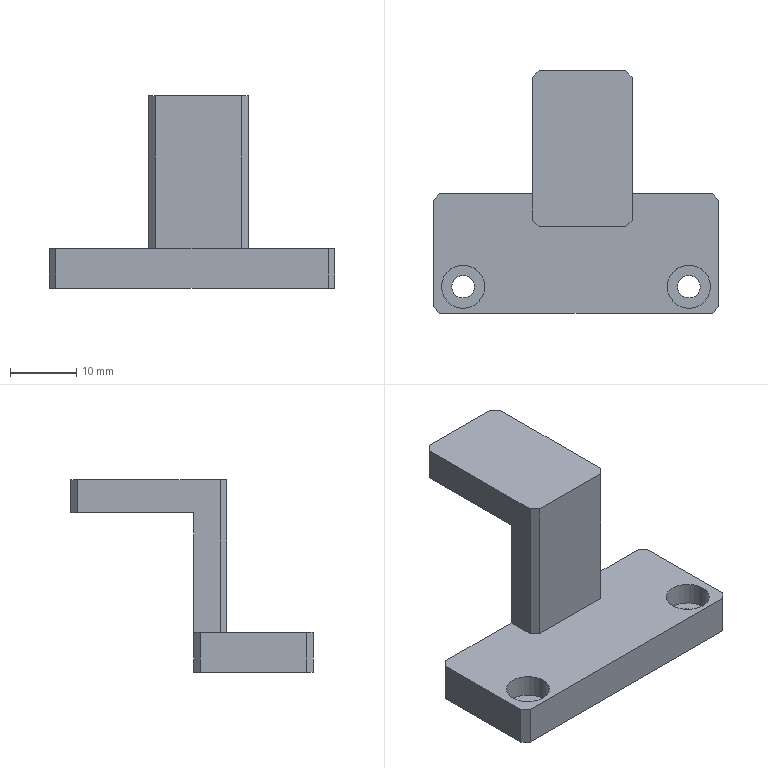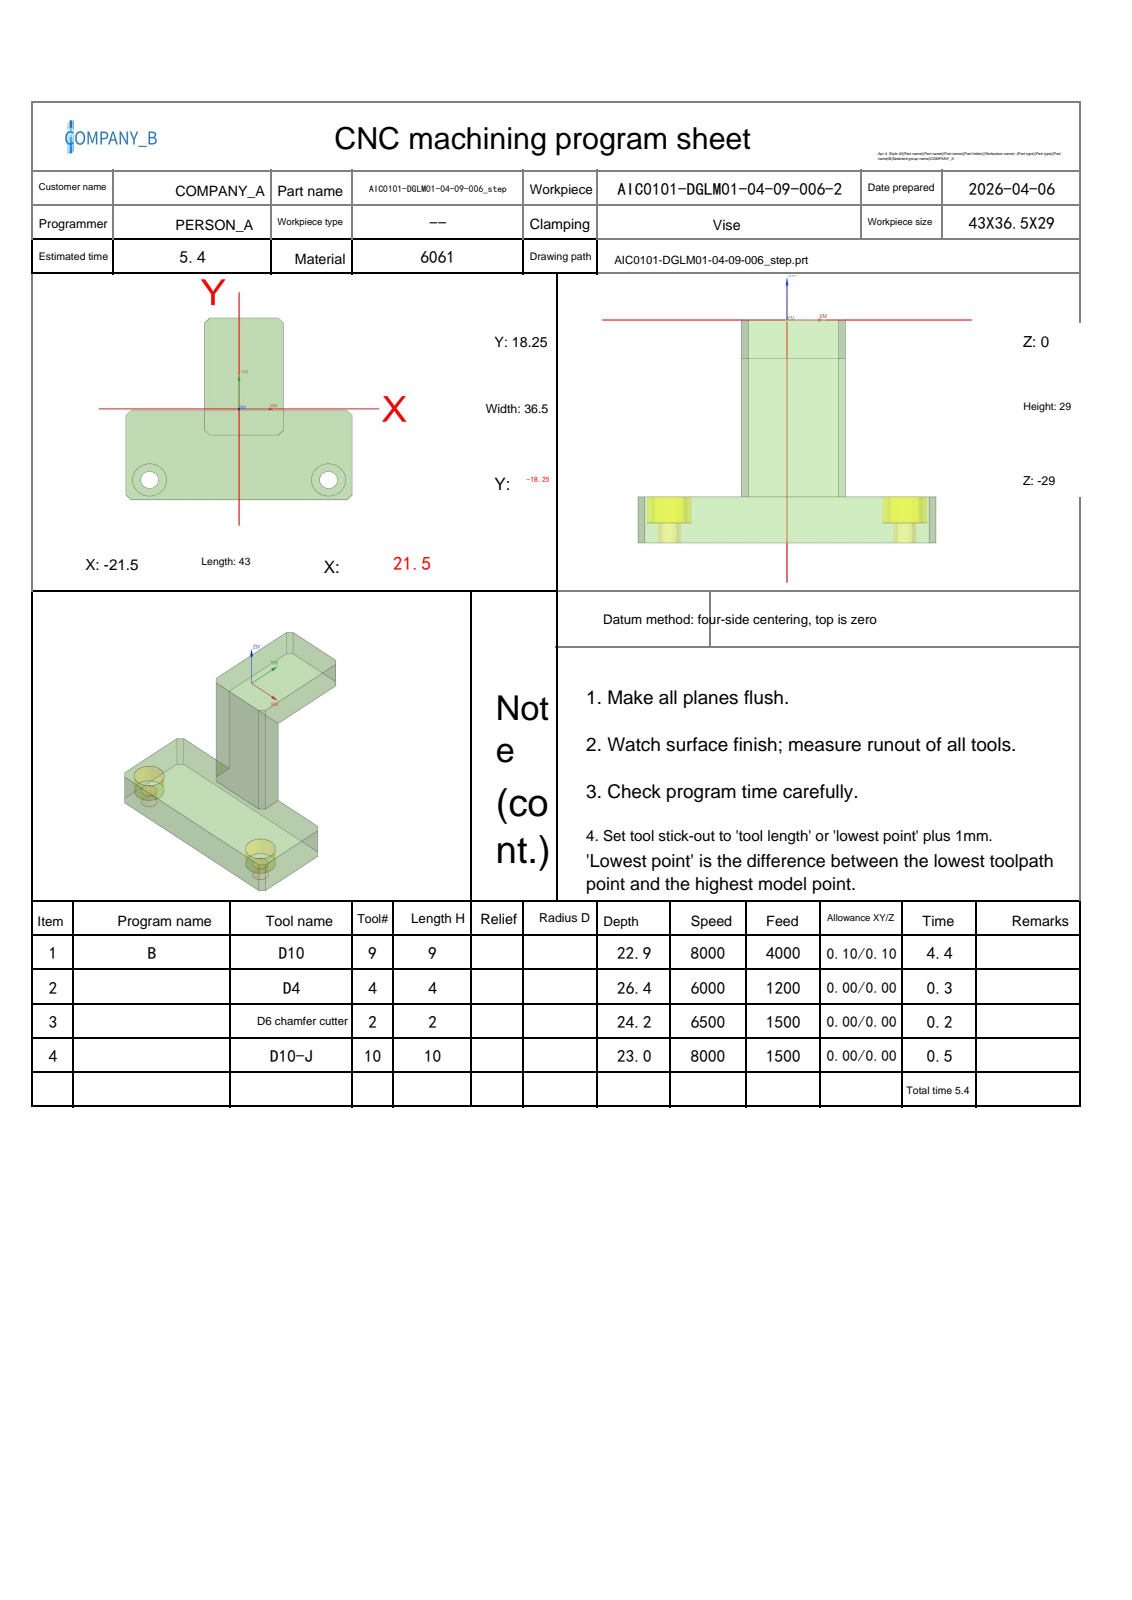NC program | NX | posted by the shop | part box 43 x 36.5 x 29 mm
Lines 4227 to 4586 of 4586:
N2 T04 M06
(D4  D=4. R=0. H=04 ce=0.07 di=0.00)
G00 G90 G54 X17. Y-14.25 M03 S6000
G43 H04 Z20.
M08
Z-22.7
G03 X17.59 Y-14.84 I.59 J0.0 F1200.
X18.18 Y-14.25 I0.0 J.59
X18.18 Y-14.25 Z-22.9 I-1.18 J0.0
X18.18 Y-14.25 Z-23.1 I-1.18 J0.0
X18.18 Y-14.25 Z-23.3 I-1.18 J0.0
X18.18 Y-14.25 Z-23.5 I-1.18 J0.0
X18.18 Y-14.25 Z-23.7 I-1.18 J0.0
X18.18 Y-14.25 Z-23.9 I-1.18 J0.0
X18.18 Y-14.25 Z-24.1 I-1.18 J0.0
X18.18 Y-14.25 Z-24.3 I-1.18 J0.0
X18.18 Y-14.25 Z-24.5 I-1.18 J0.0
X18.18 Y-14.25 Z-24.7 I-1.18 J0.0
X18.18 Y-14.25 Z-24.9 I-1.18 J0.0
X18.18 Y-14.25 Z-25.1 I-1.18 J0.0
X18.18 Y-14.25 Z-25.3 I-1.18 J0.0
X18.18 Y-14.25 Z-25.5 I-1.18 J0.0
X18.18 Y-14.25 Z-25.7 I-1.18 J0.0
X18.18 Y-14.25 Z-25.9 I-1.18 J0.0
X18.18 Y-14.25 Z-26.1 I-1.18 J0.0
X18.18 Y-14.25 Z-26.3 I-1.18 J0.0
X15.82 Y-14.25 Z-26.4 I-1.18 J0.0
X17. Y-15.43 I1.18 J0.0
X18.18 Y-14.25 I0.0 J1.18
X17. Y-13.07 I-1.18 J0.0
X15.82 Y-14.25 I0.0 J-1.18
X16.41 Y-14.84 I.59 J0.0
X17. Y-14.25 I0.0 J.59
G00 Z20.
X-17.
Z-22.7
G03 X-16.41 Y-14.84 I.59 J0.0
X-15.82 Y-14.25 I0.0 J.59
X-15.82 Y-14.25 Z-22.9 I-1.18 J0.0
X-15.82 Y-14.25 Z-23.1 I-1.18 J0.0
X-15.82 Y-14.25 Z-23.3 I-1.18 J0.0
X-15.82 Y-14.25 Z-23.5 I-1.18 J0.0
X-15.82 Y-14.25 Z-23.7 I-1.18 J0.0
X-15.82 Y-14.25 Z-23.9 I-1.18 J0.0
X-15.82 Y-14.25 Z-24.1 I-1.18 J0.0
X-15.82 Y-14.25 Z-24.3 I-1.18 J0.0
X-15.82 Y-14.25 Z-24.5 I-1.18 J0.0
X-15.82 Y-14.25 Z-24.7 I-1.18 J0.0
X-15.82 Y-14.25 Z-24.9 I-1.18 J0.0
X-15.82 Y-14.25 Z-25.1 I-1.18 J0.0
X-15.82 Y-14.25 Z-25.3 I-1.18 J0.0
X-15.82 Y-14.25 Z-25.5 I-1.18 J0.0
X-15.82 Y-14.25 Z-25.7 I-1.18 J0.0
X-15.82 Y-14.25 Z-25.9 I-1.18 J0.0
X-15.82 Y-14.25 Z-26.1 I-1.18 J0.0
X-15.82 Y-14.25 Z-26.3 I-1.18 J0.0
X-18.18 Y-14.25 Z-26.4 I-1.18 J0.0
X-17. Y-15.43 I1.18 J0.0
X-15.82 Y-14.25 I0.0 J1.18
X-17. Y-13.07 I-1.18 J0.0
X-18.18 Y-14.25 I0.0 J-1.18
X-17.59 Y-14.84 I.59 J0.0
X-17. Y-14.25 I0.0 J.59
G00 Z20.
G00 G90 X17. Y-14.25 M03 S6000
Z20.
Z-26.4
G01 X17.828 Y-14.547 F600.
X17.935 Y-14.565
G03 X18.25 Y-14.25 I0.0 J.315
X17. Y-13. I-1.25 J0.0
X15.75 Y-14.25 I0.0 J-1.25
X17. Y-15.5 I1.25 J0.0
X18.25 Y-14.25 I0.0 J1.25
X18.151 Y-13.763 I-1.25 J0.0
X17.861 Y-13.571 I-.29 J-.123
X17.647 Y-13.654 I0.0 J-.315
G01 X17. Y-14.25
G00 Z20.
X-17.
Z-26.4
G01 X-16.172 Y-14.547
X-16.065 Y-14.565
G03 X-15.75 Y-14.25 I0.0 J.315
X-17. Y-13. I-1.25 J0.0
X-18.25 Y-14.25 I0.0 J-1.25
X-17. Y-15.5 I1.25 J0.0
X-15.75 Y-14.25 I0.0 J1.25
X-15.849 Y-13.763 I-1.25 J0.0
X-16.139 Y-13.571 I-.29 J-.123
X-16.353 Y-13.654 I0.0 J-.315
G01 X-17. Y-14.25
G00 Z20.
G91 G28 Z0.0
M05
M09
G91 G28 Z0.0
M01
N3 T02 M06
(D6 chamfer cutter  D=6. R=0. H=02 ce=0.00 di=0.00)
G00 G90 G54 X9.677 Y6.886 M03 S6500
G43 H02 Z20.
M08
Z.172
G01 Z-1.2 F1500.
G03 X9.477 Y6.6 I1.532 J-1.286
G01 X9.447 Y6.554
X9.45 Y6.5
Y-4.25
X9.416 Y-4.509
X9.316 Y-4.75
X9.157 Y-4.957
X8.157 Y-5.957
X7.95 Y-6.116
X7.709 Y-6.216
X7.45 Y-6.25
X-5.55
X-5.809 Y-6.216
X-6.05 Y-6.116
X-6.257 Y-5.957
X-7.257 Y-4.957
X-7.416 Y-4.75
X-7.516 Y-4.509
X-7.55 Y-4.25
Y17.25
X-7.516 Y17.509
X-7.416 Y17.75
X-7.257 Y17.957
X-6.257 Y18.957
X-6.05 Y19.116
X-5.809 Y19.216
X-5.55 Y19.25
X7.45
X7.709 Y19.216
X7.95 Y19.116
X8.157 Y18.957
X9.157 Y17.957
X9.316 Y17.75
X9.416 Y17.509
X9.45 Y17.25
Y6.5
X9.447 Y6.446
X9.477 Y6.4
G03 X9.677 Y6.114 I1.732 J1.
G01 Z.172
G00 Z10.
X11.668 Y.795
Z-1.819
G01 Z-24.2
X11.725 Y.755
X11.745 Y.75
X20.5
X20.759 Y.716
X21. Y.616
X21.207 Y.457
X22.207 Y-.543
X22.366 Y-.75
X22.466 Y-.991
X22.5 Y-1.25
Y-17.25
X22.466 Y-17.509
X22.366 Y-17.75
X22.207 Y-17.957
X21.207 Y-18.957
X21. Y-19.116
X20.759 Y-19.216
X20.5 Y-19.25
X-20.5
X-20.759 Y-19.216
X-21. Y-19.116
X-21.207 Y-18.957
X-22.207 Y-17.957
X-22.366 Y-17.75
X-22.466 Y-17.509
X-22.5 Y-17.25
Y-1.25
X-22.466 Y-.991
X-22.366 Y-.75
X-22.207 Y-.543
X-21.207 Y.457
X-21. Y.616
X-20.759 Y.716
X-20.5 Y.75
X-9.821
X-9.801 Y.755
X-9.744 Y.795
Z-1.795
G00 Z10.
X-19.058 Y-13.846
Z-22.747
G01 Z-24.2
G03 X-19.232 Y-14.148 I1.638 J-1.147
G01 X-19.258 Y-14.196
X-19.25 Y-14.25
G03 X-17. Y-16.5 I2.25 J0.0
X-14.75 Y-14.25 I0.0 J2.25
X-17. Y-12. I-2.25 J0.0
X-19.25 Y-14.25 I0.0 J-2.25
G01 X-19.258 Y-14.304
X-19.232 Y-14.352
G03 X-19.058 Y-14.654 I1.813 J.845
G01 Z-22.747
G00 Z10.
X14.942 Y-13.846
Z-22.747
G01 Z-24.2
G03 X14.768 Y-14.148 I1.638 J-1.147
G01 X14.742 Y-14.196
X14.75 Y-14.25
G03 X17. Y-16.5 I2.25 J0.0
X19.25 Y-14.25 I0.0 J2.25
X17. Y-12. I-2.25 J0.0
X14.75 Y-14.25 I0.0 J-2.25
G01 X14.742 Y-14.304
X14.768 Y-14.352
G03 X14.942 Y-14.654 I1.813 J.845
G01 Z-22.747
G00 Z20.
G91 G28 Z0.0
M05
M09
G91 G28 Z0.0
M01
N4 T10 M06
(D10-J  D=10. R=0. H=10 ce=0.40 di=0.00)
G00 G90 G54 X-8.585 Y-12.002 M03 S7000
G43 H10 Z15.5
M08
Z1.5
G01 Z0.0 F1500.
G03 X-7.55 Y-10.25 I-.964 J1.752
G01 Y22.35
G02 X-6.65 Y23.25 I.9 J0.0
G01 X-4.55
G02 X-3.55 Y22.25 I0.0 J-1.
G01 Y-9.35
G03 X-2.65 Y-10.25 I.9 J0.0
G01 X-.55
G03 X.45 Y-9.25 I0.0 J1.
G01 Y22.35
G02 X1.35 Y23.25 I.9 J0.0
G01 X3.45
G02 X4.45 Y22.25 I0.0 J-1.
G01 Y-10.25
G02 X2.45 Y-12.25 I-2. J0.0
G01 Z1.5
G00 Z15.5
G00 G90 X-28.071 Y-19.892 M03 S7000
Z15.5
Z-21.5
G01 Z-23. F1500.
X-25.328 Y-17.15
G02 X-23.914 Y-16.564 I1.414 J-1.414
X-22.5 Y-17.15 I0.0 J-2.
G01 X-20.648 Y-19.002
G03 X-20.049 Y-19.25 I.6 J.6
G01 X-13.886
G03 X-13.586 Y-18.95 I0.0 J.3
X-13.708 Y-18.708 I-.3 J0.0
G02 X-14.858 Y-17.721 I5.921 J8.058
G01 X-19.021 Y-13.558
G02 X-21.95 Y-6.487 I7.071 J7.071
G01 Y-.286
G03 X-23.95 Y1.714 I-2. J0.0
G01 X-27.931
Z-21.5
G00 Z15.5
X28.5 Y-12.673
Z-21.5
G01 Z-23.
X25.234 Y-10.778
G03 X24.23 Y-10.508 I-1.004 J-1.73
X22.5 Y-11.504 I0.0 J-2.
G02 X20.921 Y-13.558 I-8.65 J5.018
G01 X16.758 Y-17.721
G02 X14.79 Y-19.25 I-7.071 J7.071
G03 X13.81 Y-20.97 I1.021 J-1.72
X14.09 Y-21.991 I2. J0.0
G01 X16.024 Y-25.25
Z-21.5
G00 Z15.5
X-18.95 Y6.75
Z-21.5
G01 Z-23.
Y2.75
G02 X-16.95 Y.75 I0.0 J-2.
G01 Y-6.487
G03 X-15.486 Y-10.022 I5. J0.0
G01 X-11.322 Y-14.186
G03 X-7.787 Y-15.65 I3.536 J3.536
G01 X9.687
G03 X13.222 Y-14.186 I0.0 J5.
G01 X17.386 Y-10.022
G03 X18.85 Y-6.487 I-3.536 J3.536
G01 Y-.024
G03 X18.1 Y.944 I-1. J0.0
G01 X15.1 Y1.718
G03 X14.85 Y1.75 I-.25 J-.968
X13.85 Y.75 I0.0 J-1.
G01 Y-6.487
X9.687 Y-10.65
X-7.787
X-11.95 Y-6.487
Y.75
G03 X-13.95 Y2.75 I-2. J0.0
G01 Y6.75
Z-21.5
G00 Z15.5
G00 G90 X15.65 Y6.75 M03 S8000
Z15.5
Z-6.667
G01 Z-7.667 F1000.
G41 D10
X15.45
G03 X13.45 Y4.75 I0.0 J-2.
G01 Y-6.321
X9.521 Y-10.25
X-7.621
X-11.55 Y-6.321
Y4.75
G03 X-13.55 Y6.75 I-2. J0.0
G01 G40 X-13.75
Z-6.667
G00 Z15.5
X15.65
Z-14.333
G01 Z-15.333
G41 D10
X15.45
G03 X13.45 Y4.75 I0.0 J-2.
G01 Y-6.321
X9.521 Y-10.25
X-7.621
X-11.55 Y-6.321
Y4.75
G03 X-13.55 Y6.75 I-2. J0.0
G01 G40 X-13.75
Z-14.333
G00 Z15.5
X15.65
Z-22.
G01 Z-23.
G41 D10
X15.45
G03 X13.45 Y4.75 I0.0 J-2.
G01 Y-6.321
X9.521 Y-10.25
X-7.621
X-11.55 Y-6.321
Y4.75
G03 X-13.55 Y6.75 I-2. J0.0
G01 G40 X-13.75
Z-22.
G00 Z15.5
M05
M09
G91 G28 Z0.0
G91 G28 Y0.0
M30
%